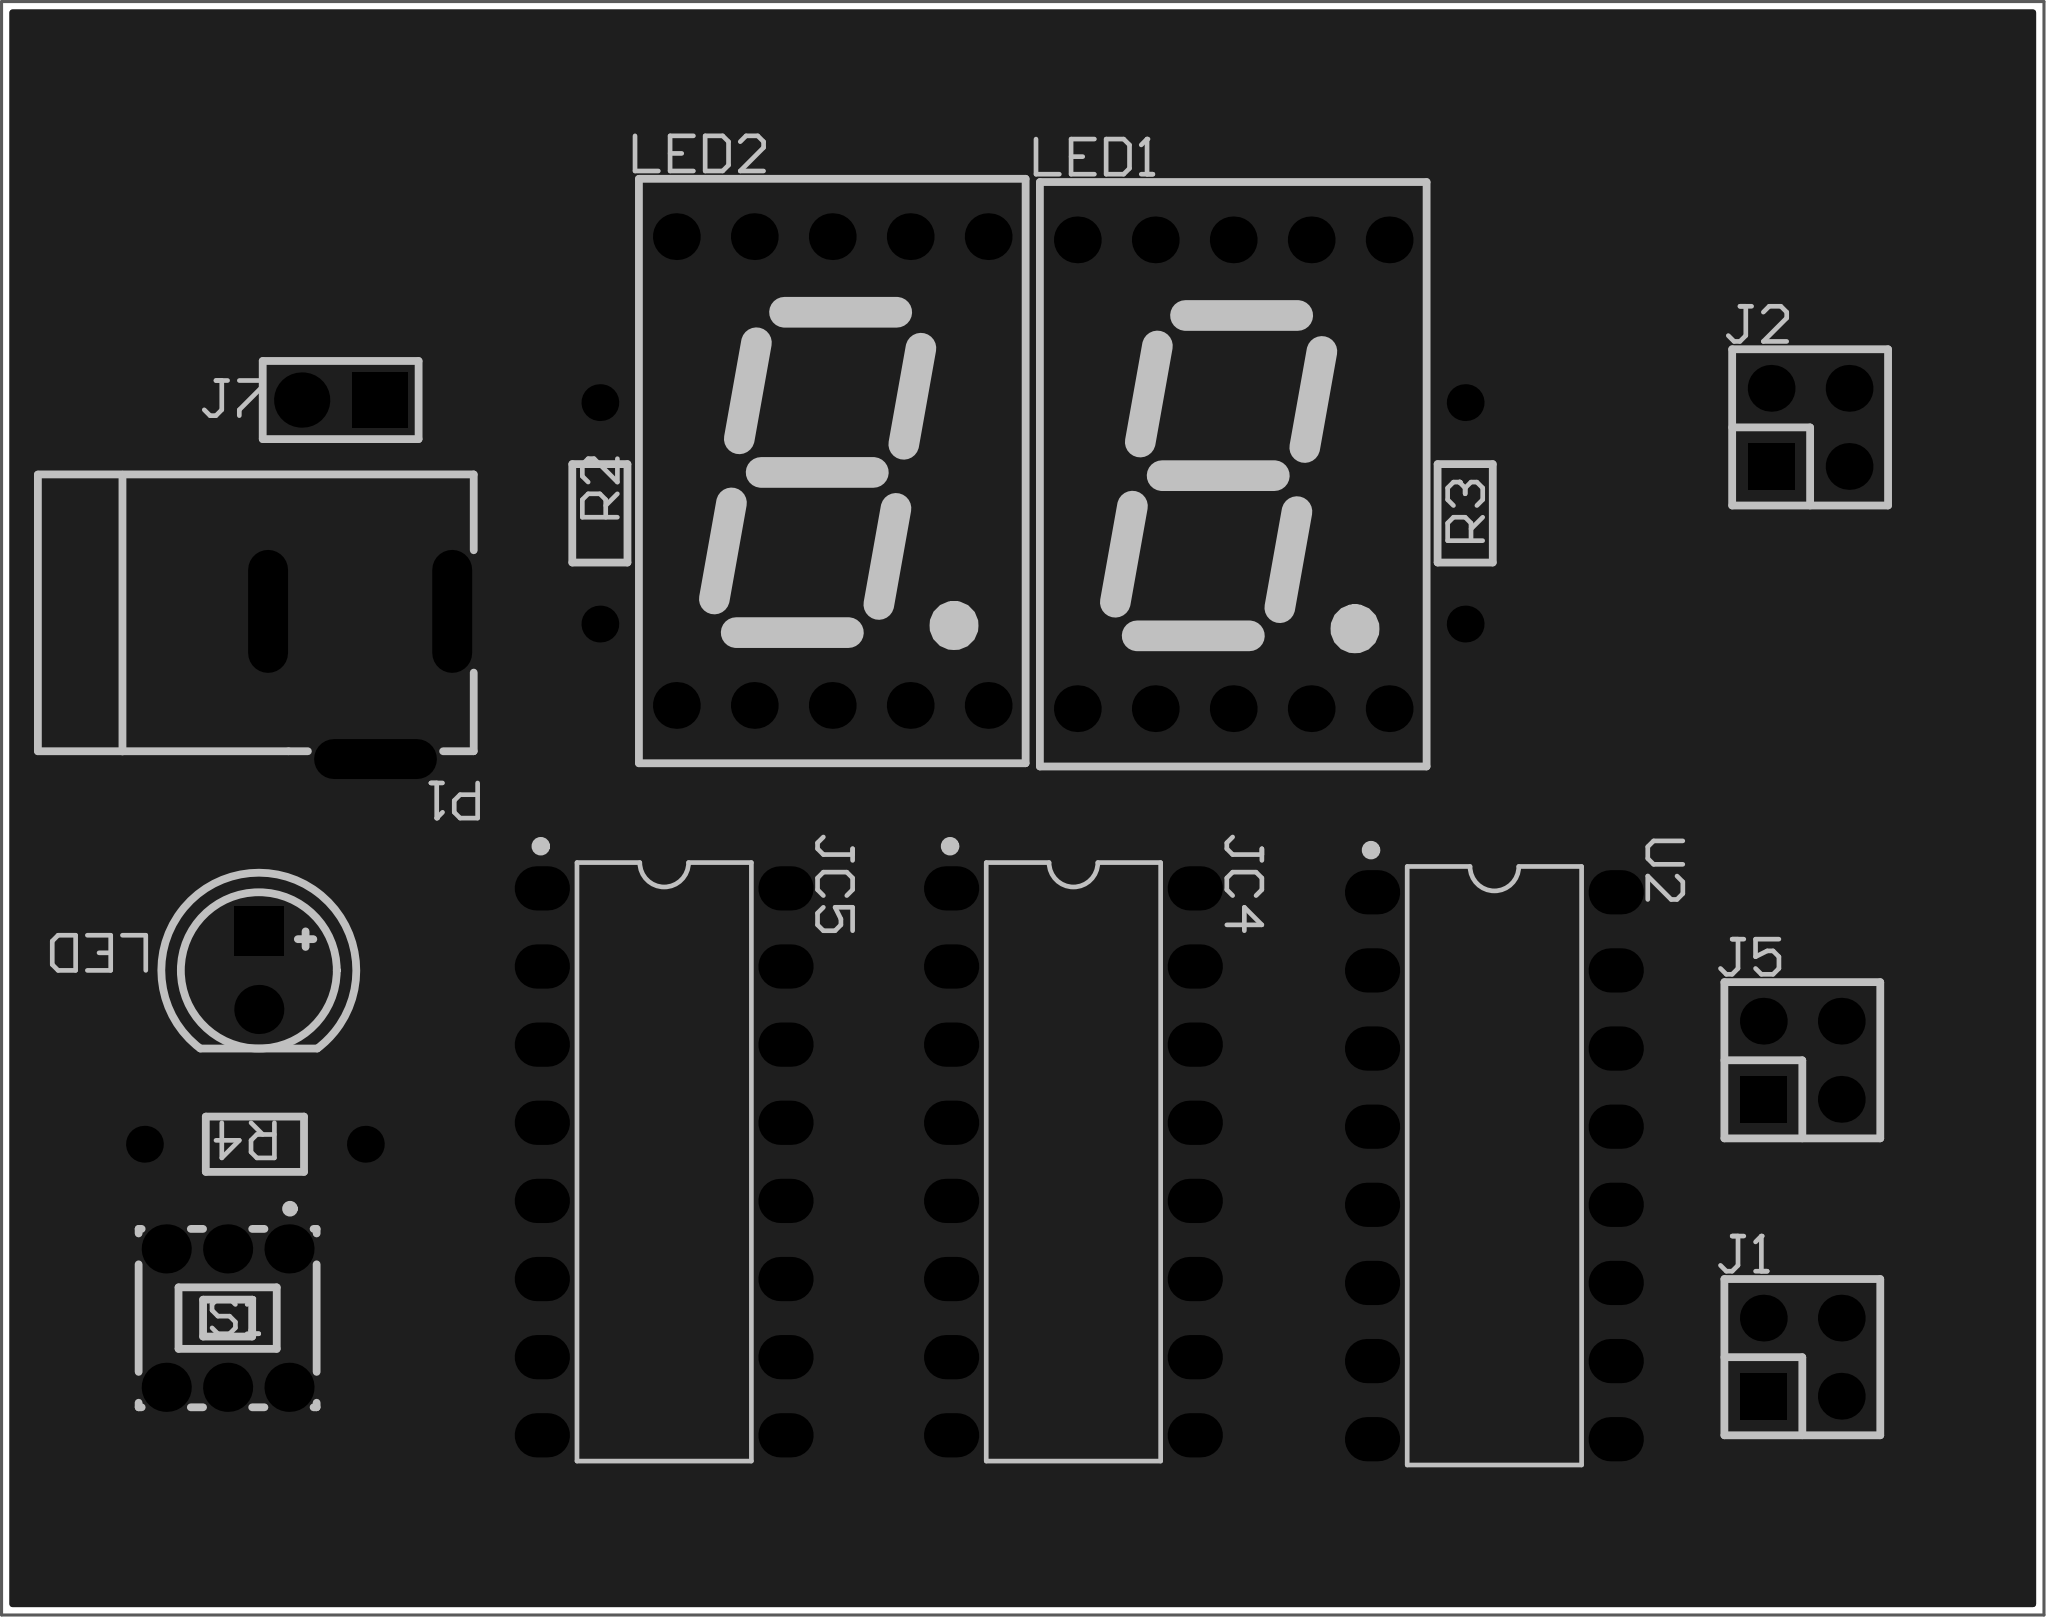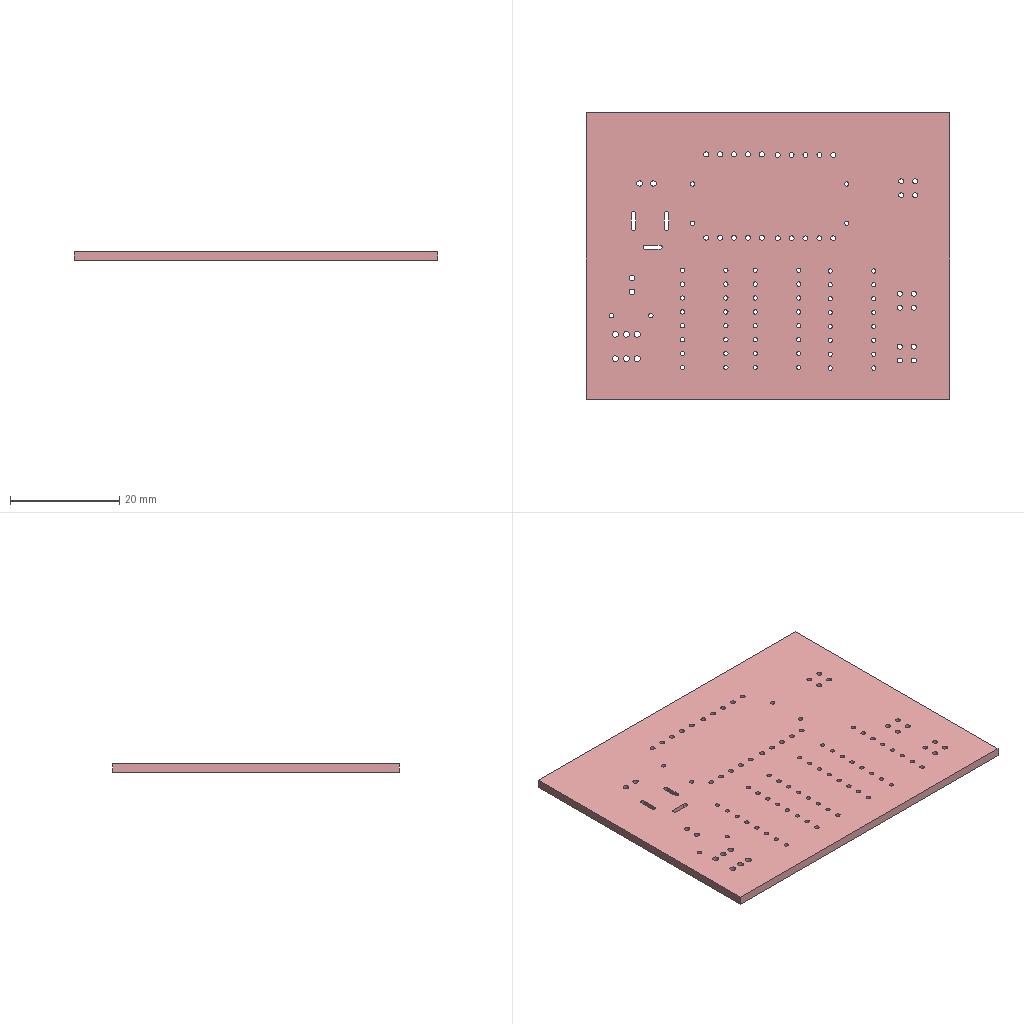Circuit board layout | Altium Designer | box 66.5 x 52.5 x 1.6 mm
Layer stack:
# Altium Designer layer stack of  (unit mm; dielectric type: 0 none, 1 core, 2 prepreg, 3 surface material)
index,name,kind,layer,copper_thickness_mm,dielectric_type,dielectric_thickness_mm,dielectric_material,dielectric_constant
0,Top Paste Mask Layer,other,,,,,,
1,Top Silkscreen Layer,other,,,,,,
2,Top Solder Mask Layer,dielectric,,,3,0.01,,3.3
3,Top Layer,copper,Top Layer,0.035,,,,
4,Dielectric1,dielectric,,,3,1.51,FR4,4.5
5,Bottom Layer,copper,Bottom Layer,0.035,,,,
6,Bottom Solder Mask Layer,dielectric,,,3,0.01,,3.3
7,Bottom Silkscreen Layer,other,,,,,,
8,Bottom Paste Mask Layer,other,,,,,,
# drill layer pairs: low layer,high layer
drill_pair,Top Layer,Bottom Layer
Part placement:
Designator,Comment,Layer,Footprint,Center-X(mm),Center-Y(mm),Rotation
P1,,TopLayer,DC-2.0,90.805,108.712,180
J2,,TopLayer,HDR-TH_4P-P2.54-V-M-R2-C2-S2.54-1,138.049,117.094,0
J5,,TopLayer,HDR-TH_4P-P2.54-V-M-R2-C2-S2.54-1,137.795,96.52,0
J1,,TopLayer,HDR-TH_4P-P2.54-V-M-R2-C2-S2.54-1,137.795,86.868,0
J7,,TopLayer,HDR-TH_2P-P2.54-V-M-1,90.17,117.983,180
LED2,,TopLayer,LED-SEG-TH_10P-L12.6-W19.0-P2.54-S15.24-BL,106.188,115.675,0
LED1,,TopLayer,LED-SEG-TH_10P-L12.6-W19.0-P2.54-S15.24-BL,119.253,115.57,0
LED,,TopLayer,LED-TH_5mm,87.503,99.441,270
R2,1kΩ,TopLayer,Res_1/8W,98.616,114.3,90
R3,1kΩ,TopLayer,Res_1/8W,126.81,114.3,90
JC5,CD74HCT4511E,TopLayer,PDIP-16_L19.3-W6.4-P2.54-LS7.94-BL,100.711,93.218,270
U2,4518BDM,TopLayer,PDIP-16_L19.3-W6.4-P2.54-LS7.94-BL,127.762,93.091,270
JC4,CD74HCT4511E,TopLayer,PDIP-16_L19.3-W6.4-P2.54-LS7.94-BL,114.046,93.218,270
S1,自锁开关 5.8Z白灰白260G,TopLayer,SW-TH_6P-L5.8-W5.8-P2.00-LS4.5-TR,86.487,88.138,0
R4,1kΩ,TopLayer,Res_1/8W,87.376,93.79,180
Pad and via stacks:
# Altium Designer via and pad stacks of  (unit mm). Each distinct definition once, with the count of objects using it.
# via: kind,start_layer,end_layer,hole_mm,diameter_mm,mode(0 simple;1 top-mid-bottom;2 full stack),diameter_per_layer,count,example_net
# pad: kind,layer,hole_mm,hole_type(0 round;1 square;2 slot),plating,top_size,top_shape(1 round;2 rect;3 octagon;9 rounded rect),mid_size,bottom_size,mode,footprint,size_per_layer,count,example
pad,Multi-Layer,0.8001,2,plated,4x1.3,1,4x1.3,4x1.3,0,DC-2.0,,3,P1.2
pad,Multi-Layer,0.9144,0,plated,1.524x1.524,2,1.524x1.524,1.524x1.524,0,HDR-TH_4P-P2.54-V-M-R2-C2-S2.54-1,,3,J2.1
pad,Multi-Layer,0.9144,0,plated,1.524x1.524,1,1.524x1.524,1.524x1.524,0,HDR-TH_4P-P2.54-V-M-R2-C2-S2.54-1,,9,J2.2
pad,Multi-Layer,1,0,plated,1.8x1.8,1,1.8x1.8,1.8x1.8,0,HDR-TH_2P-P2.54-V-M-1,,1,J7.2
pad,Multi-Layer,1,0,plated,1.8x1.8,2,1.8x1.8,1.8x1.8,0,HDR-TH_2P-P2.54-V-M-1,,1,J7.1
pad,Multi-Layer,0.9144,0,plated,1.524x1.524,1,1.524x1.524,1.524x1.524,0,LED-SEG-TH_10P-L12.6-W19.0-P2.54-S15.24-BL,,20,LED2.1
pad,Multi-Layer,1,0,plated,1.6x1.6,2,1.6x1.6,1.6x1.6,0,LED-TH_5mm,,1,LED.1
pad,Multi-Layer,1,0,plated,1.6x1.6,1,1.6x1.6,1.6x1.6,0,LED-TH_5mm,,1,LED.2
pad,Multi-Layer,0.8001,0,plated,1.199x1.199,1,1.199x1.199,1.199x1.199,0,Res_1/8W,,6,R2.1
pad,Multi-Layer,0.8,0,plated,1.44x1.8,1,1.44x1.8,1.44x1.8,0,PDIP-16_L19.3-W6.4-P2.54-LS7.94-BL,,48,JC5.1
pad,Multi-Layer,1.1,0,plated,1.6x1.6,1,1.6x1.6,1.6x1.6,0,SW-TH_6P-L5.8-W5.8-P2.00-LS4.5-TR,,6,S1.6
Copper pours:
name,layer,net,type(0 solid;1 hatched;2 none)
Top Layer-GND,Top Layer,GND,0
Bottom Layer-GND,Bottom Layer,GND,0